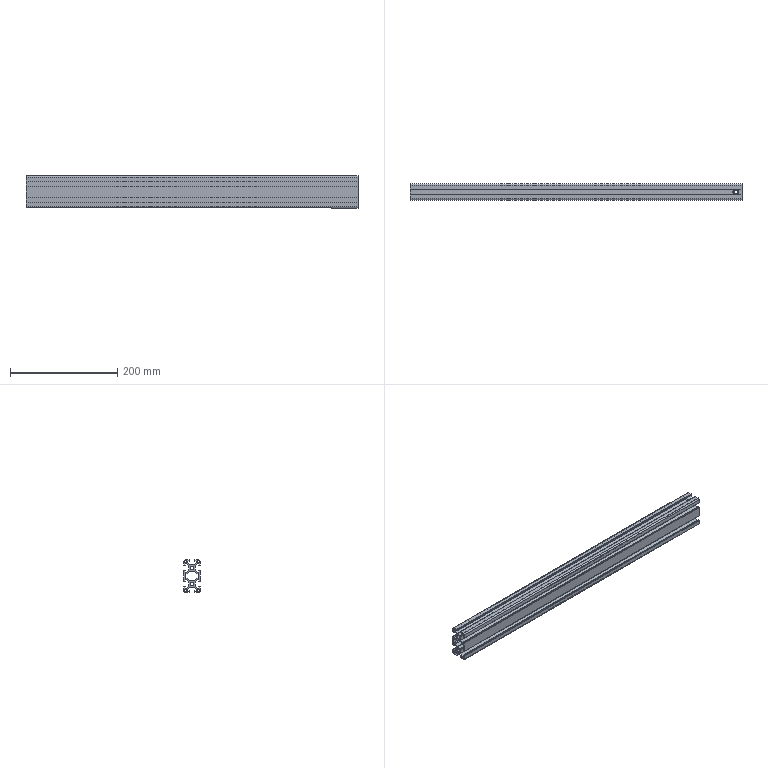Part | STEP file | 1 solid | 282 faces | box 620 x 30 x 60.001 mm | volume 358896 mm3 | cylinder 150 | plane 128 | cone 4 | commonest cylinder face diameters 0.6 x94 2 x32 6.8 x6 11 x6 5 x4 6.6 x4